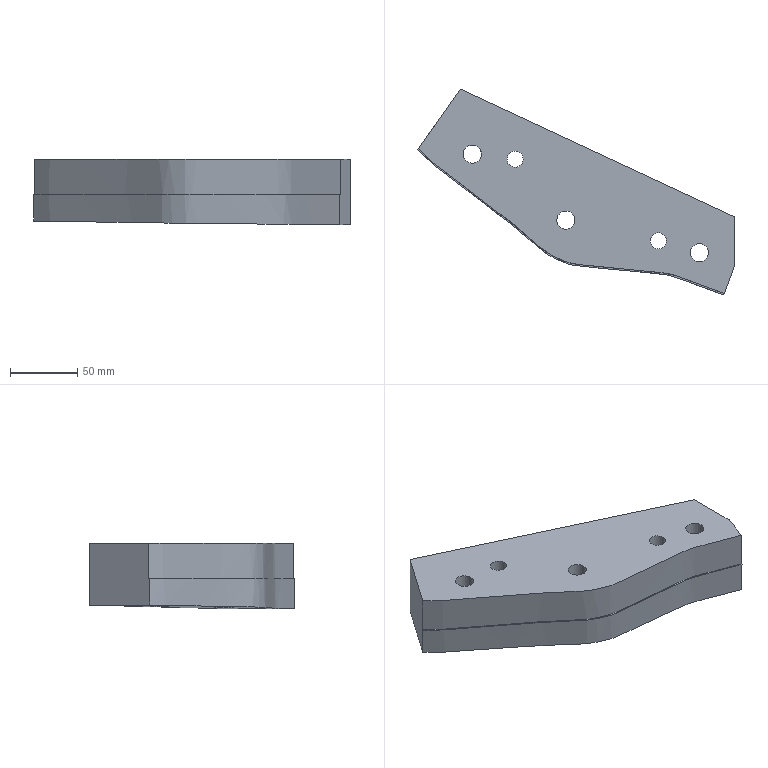Part | NX | features solid 2 | 1 solid | 24 faces | box 234.961 x 152.688 x 48.86 mm | volume 747452 mm3 | plane 12 | cylinder 10 | spline 2 | commonest cylinder face diameters 13.5 x3 19.5 x3 12 x2 13 x2
STEP:
#1=CARTESIAN_POINT('',(-144.165,133.045,40.));
#2=VERTEX_POINT('',#1);
#3=CARTESIAN_POINT('',(-150.915,133.045,40.));
#4=DIRECTION('',(0.,0.,1.));
#5=DIRECTION('',(1.,0.,0.));
#6=AXIS2_PLACEMENT_3D('',#3,#4,#5);
#7=CIRCLE('',#6,6.75);
#8=EDGE_CURVE('',#2,#2,#7,.T.);
#9=ORIENTED_EDGE('',*,*,#8,.F.);
#10=EDGE_LOOP('',(#9));
#11=FACE_BOUND('',#10,.T.);
#12=CARTESIAN_POINT('',(-312.729,206.131,40.));
#13=VERTEX_POINT('',#12);
#14=CARTESIAN_POINT('',(-319.479,206.131,40.));
#15=DIRECTION('',(0.,0.,1.));
#16=DIRECTION('',(1.,0.,0.));
#17=AXIS2_PLACEMENT_3D('',#14,#15,#16);
#18=CIRCLE('',#17,6.75);
#19=EDGE_CURVE('',#13,#13,#18,.T.);
#20=ORIENTED_EDGE('',*,*,#19,.F.);
#21=EDGE_LOOP('',(#20));
#22=FACE_BOUND('',#21,.T.);
#23=CARTESIAN_POINT('',(-243.241,157.177,40.));
#24=VERTEX_POINT('',#23);
#25=CARTESIAN_POINT('',(-249.991,157.177,40.));
#26=DIRECTION('',(0.,0.,1.));
#27=DIRECTION('',(1.,0.,0.));
#28=AXIS2_PLACEMENT_3D('',#25,#26,#27);
#29=CIRCLE('',#28,6.75);
#30=EDGE_CURVE('',#24,#24,#29,.T.);
#31=ORIENTED_EDGE('',*,*,#30,.F.);
#32=EDGE_LOOP('',(#31));
#33=FACE_BOUND('',#32,.T.);
#34=CARTESIAN_POINT('',(-175.436,141.76,40.));
#35=VERTEX_POINT('',#34);
#36=CARTESIAN_POINT('',(-181.436,141.76,40.));
#37=DIRECTION('',(0.,0.,1.));
#38=DIRECTION('',(1.,0.,0.));
#39=AXIS2_PLACEMENT_3D('',#36,#37,#38);
#40=CIRCLE('',#39,6.);
#41=EDGE_CURVE('',#35,#35,#40,.T.);
#42=ORIENTED_EDGE('',*,*,#41,.F.);
#43=EDGE_LOOP('',(#42));
#44=FACE_BOUND('',#43,.T.);
#45=CARTESIAN_POINT('',(-281.644,202.32,40.));
#46=VERTEX_POINT('',#45);
#47=CARTESIAN_POINT('',(-287.644,202.32,40.));
#48=DIRECTION('',(0.,0.,1.));
#49=DIRECTION('',(1.,0.,0.));
#50=AXIS2_PLACEMENT_3D('',#47,#48,#49);
#51=CIRCLE('',#50,6.);
#52=EDGE_CURVE('',#46,#46,#51,.T.);
#53=ORIENTED_EDGE('',*,*,#52,.F.);
#54=EDGE_LOOP('',(#53));
#55=FACE_BOUND('',#54,.T.);
#56=CARTESIAN_POINT('',(-132.408,102.674,40.));
#57=VERTEX_POINT('',#56);
#58=CARTESIAN_POINT('',(-359.384,210.162,40.));
#59=VERTEX_POINT('',#58);
#60=CARTESIAN_POINT('',(-132.408,102.674,40.));
#61=CARTESIAN_POINT('',(-133.704,103.14,40.));
#62=CARTESIAN_POINT('',(-136.335,104.003,40.));
#63=CARTESIAN_POINT('',(-141.52,105.911,40.));
#64=CARTESIAN_POINT('',(-147.98,108.359,40.));
#65=CARTESIAN_POINT('',(-155.752,111.253,40.));
#66=CARTESIAN_POINT('',(-163.506,114.139,40.));
#67=CARTESIAN_POINT('',(-171.267,117.226,40.));
#68=CARTESIAN_POINT('',(-179.47,118.263,40.));
#69=CARTESIAN_POINT('',(-187.623,119.24,40.));
#70=CARTESIAN_POINT('',(-195.819,119.959,40.));
#71=CARTESIAN_POINT('',(-204.02,120.604,40.));
#72=CARTESIAN_POINT('',(-212.219,121.277,40.));
#73=CARTESIAN_POINT('',(-220.405,122.065,40.));
#74=CARTESIAN_POINT('',(-228.561,123.135,40.));
#75=CARTESIAN_POINT('',(-235.386,123.797,40.));
#76=CARTESIAN_POINT('',(-240.845,124.247,40.));
#77=CARTESIAN_POINT('',(-244.943,124.767,40.));
#78=CARTESIAN_POINT('',(-248.867,125.792,40.));
#79=CARTESIAN_POINT('',(-252.61,127.306,40.));
#80=CARTESIAN_POINT('',(-256.299,128.954,40.));
#81=CARTESIAN_POINT('',(-259.983,130.668,40.));
#82=CARTESIAN_POINT('',(-263.483,132.667,40.));
#83=CARTESIAN_POINT('',(-266.659,135.061,40.));
#84=CARTESIAN_POINT('',(-269.686,137.645,40.));
#85=CARTESIAN_POINT('',(-272.75,140.183,40.));
#86=CARTESIAN_POINT('',(-275.752,142.798,40.));
#87=CARTESIAN_POINT('',(-279.678,146.382,40.));
#88=CARTESIAN_POINT('',(-284.663,150.764,40.));
#89=CARTESIAN_POINT('',(-290.913,155.686,40.));
#90=CARTESIAN_POINT('',(-299.232,162.266,40.));
#91=CARTESIAN_POINT('',(-309.703,170.4,40.));
#92=CARTESIAN_POINT('',(-320.302,178.373,40.));
#93=CARTESIAN_POINT('',(-328.787,184.744,40.));
#94=CARTESIAN_POINT('',(-335.144,189.531,40.));
#95=CARTESIAN_POINT('',(-341.443,194.391,40.));
#96=CARTESIAN_POINT('',(-346.778,198.333,40.));
#97=CARTESIAN_POINT('',(-350.821,201.768,40.));
#98=CARTESIAN_POINT('',(-354.614,205.514,40.));
#99=CARTESIAN_POINT('',(-357.386,208.414,40.));
#100=CARTESIAN_POINT('',(-359.384,210.162,40.));
#101=B_SPLINE_CURVE_WITH_KNOTS('',3,(#60,#61,#62,#63,#64,#65,#66,#67,#68,#69,#70,#71,#72,#73,#74,#75,#76,#77,#78,#79,#80,#81,#82,#83,#84,#85,#86,#87,#88,#89,#90,#91,#92,#93,#94,#95,#96,#97,#98,#99,#100),.UNSPECIFIED.,.F.,.F.,(4,1,1,1,1,1,1,1,1,1,1,1,1,1,1,1,1,1,1,1,1,1,1,1,1,1,1,1,1,1,1,1,1,1,1,1,1,1,4),(0.01102,0.01506,0.0191,0.02717,0.03525,0.04332,0.0514,0.05947,0.06755,0.07562,0.0837,0.09177,0.09985,0.1079,0.116,0.12,0.1241,0.1281,0.1322,0.1362,0.1402,0.1443,0.1483,0.1523,0.1564,0.1604,0.1645,0.1725,0.1806,0.1887,0.2048,0.221,0.2291,0.2371,0.2452,0.2533,0.2573,0.2614,0.2694),.UNSPECIFIED.);
#102=EDGE_CURVE('',#57,#59,#101,.T.);
#103=ORIENTED_EDGE('',*,*,#102,.F.);
#104=CARTESIAN_POINT('',(-125.,123.027,40.));
#105=VERTEX_POINT('',#104);
#106=CARTESIAN_POINT('',(-187.242,-47.981,40.));
#107=DIRECTION('',(0.342,0.9397,0.));
#108=VECTOR('',#107,1000.);
#109=LINE('',#106,#108);
#110=EDGE_CURVE('',#57,#105,#109,.T.);
#111=ORIENTED_EDGE('',*,*,#110,.T.);
#112=CARTESIAN_POINT('',(-125.,159.579,40.));
#113=VERTEX_POINT('',#112);
#114=CARTESIAN_POINT('',(-125.,35.09,40.));
#115=DIRECTION('',(0.,1.,0.));
#116=VECTOR('',#115,1000.);
#117=LINE('',#114,#116);
#118=EDGE_CURVE('',#105,#113,#117,.T.);
#119=ORIENTED_EDGE('',*,*,#118,.T.);
#120=CARTESIAN_POINT('',(-328.392,254.422,40.));
#121=VERTEX_POINT('',#120);
#122=CARTESIAN_POINT('',(-99.435,147.658,40.));
#123=DIRECTION('',(0.9063,-0.4226,0.));
#124=VECTOR('',#123,1000.);
#125=LINE('',#122,#124);
#126=EDGE_CURVE('',#113,#121,#125,.F.);
#127=ORIENTED_EDGE('',*,*,#126,.T.);
#128=CARTESIAN_POINT('',(-460.095,66.332,40.));
#129=DIRECTION('',(0.5736,0.8192,0.));
#130=VECTOR('',#129,1000.);
#131=LINE('',#128,#130);
#132=EDGE_CURVE('',#59,#121,#131,.T.);
#133=ORIENTED_EDGE('',*,*,#132,.F.);
#134=EDGE_LOOP('',(#103,#111,#119,#127,#133));
#135=FACE_BOUND('',#134,.T.);
#136=CARTESIAN_POINT('',(-415.478,35.09,40.));
#137=DIRECTION('',(0.,0.,1.));
#138=DIRECTION('',(1.,0.,0.));
#139=AXIS2_PLACEMENT_3D('',#136,#137,#138);
#140=PLANE('',#139);
#141=ADVANCED_FACE('',(#11,#22,#33,#44,#55,#135),#140,.T.);
#142=ORIENTED_EDGE('',*,*,#118,.F.);
#143=CARTESIAN_POINT('',(-125.,123.027,-8.793));
#144=VERTEX_POINT('',#143);
#145=CARTESIAN_POINT('',(-125.,123.027,23.));
#146=DIRECTION('',(0.,0.,-1.));
#147=VECTOR('',#146,1000.);
#148=LINE('',#145,#147);
#149=EDGE_CURVE('',#105,#144,#148,.T.);
#150=ORIENTED_EDGE('',*,*,#149,.T.);
#151=CARTESIAN_POINT('',(-125.,159.579,-8.551));
#152=VERTEX_POINT('',#151);
#153=CARTESIAN_POINT('',(-125.,163.829,-8.523));
#154=DIRECTION('',(0.,-1.,-0.00662));
#155=VECTOR('',#154,1000.);
#156=LINE('',#153,#155);
#157=EDGE_CURVE('',#152,#144,#156,.T.);
#158=ORIENTED_EDGE('',*,*,#157,.F.);
#159=CARTESIAN_POINT('',(-125.,159.579,2.));
#160=DIRECTION('',(0.,0.,-1.));
#161=VECTOR('',#160,1000.);
#162=LINE('',#159,#161);
#163=EDGE_CURVE('',#152,#113,#162,.F.);
#164=ORIENTED_EDGE('',*,*,#163,.T.);
#165=EDGE_LOOP('',(#142,#150,#158,#164));
#166=FACE_BOUND('',#165,.T.);
#167=CARTESIAN_POINT('',(-125.,163.62,23.));
#168=DIRECTION('',(1.,0.,0.));
#169=DIRECTION('',(0.,0.,-1.));
#170=AXIS2_PLACEMENT_3D('',#167,#168,#169);
#171=PLANE('',#170);
#172=ADVANCED_FACE('',(#166),#171,.T.);
#173=CARTESIAN_POINT('',(-359.961,209.338,-6.));
#174=VERTEX_POINT('',#173);
#175=CARTESIAN_POINT('',(-132.75,101.734,-8.86));
#176=VERTEX_POINT('',#175);
#177=CARTESIAN_POINT('',(-359.961,209.338,-6.));
#178=CARTESIAN_POINT('',(-357.935,207.556,-6.031));
#179=CARTESIAN_POINT('',(-355.147,204.621,-6.077));
#180=CARTESIAN_POINT('',(-351.299,200.848,-6.138));
#181=CARTESIAN_POINT('',(-347.183,197.387,-6.2));
#182=CARTESIAN_POINT('',(-341.764,193.377,-6.278));
#183=CARTESIAN_POINT('',(-335.365,188.443,-6.371));
#184=CARTESIAN_POINT('',(-328.907,183.583,-6.464));
#185=CARTESIAN_POINT('',(-320.289,177.113,-6.588));
#186=CARTESIAN_POINT('',(-309.528,169.009,-6.744));
#187=CARTESIAN_POINT('',(-298.9,160.735,-6.899));
#188=CARTESIAN_POINT('',(-290.451,154.045,-7.023));
#189=CARTESIAN_POINT('',(-284.11,149.034,-7.116));
#190=CARTESIAN_POINT('',(-278.12,143.567,-7.209));
#191=CARTESIAN_POINT('',(-273.048,139.115,-7.287));
#192=CARTESIAN_POINT('',(-268.899,135.674,-7.349));
#193=CARTESIAN_POINT('',(-265.799,133.078,-7.395));
#194=CARTESIAN_POINT('',(-262.422,130.844,-7.442));
#195=CARTESIAN_POINT('',(-258.768,128.97,-7.489));
#196=CARTESIAN_POINT('',(-254.985,127.275,-7.536));
#197=CARTESIAN_POINT('',(-251.21,125.617,-7.582));
#198=CARTESIAN_POINT('',(-247.364,124.283,-7.628));
#199=CARTESIAN_POINT('',(-243.399,123.523,-7.67));
#200=CARTESIAN_POINT('',(-239.361,123.116,-7.711));
#201=CARTESIAN_POINT('',(-233.956,122.673,-7.765));
#202=CARTESIAN_POINT('',(-227.235,121.95,-7.833));
#203=CARTESIAN_POINT('',(-219.201,120.928,-7.916));
#204=CARTESIAN_POINT('',(-211.135,120.181,-7.997));
#205=CARTESIAN_POINT('',(-203.059,119.526,-8.078));
#206=CARTESIAN_POINT('',(-194.982,118.887,-8.159));
#207=CARTESIAN_POINT('',(-186.909,118.159,-8.24));
#208=CARTESIAN_POINT('',(-178.885,117.187,-8.322));
#209=CARTESIAN_POINT('',(-172.138,116.282,-8.392));
#210=CARTESIAN_POINT('',(-167.026,114.447,-8.452));
#211=CARTESIAN_POINT('',(-161.971,112.515,-8.513));
#212=CARTESIAN_POINT('',(-155.633,110.135,-8.589));
#213=CARTESIAN_POINT('',(-148.018,107.308,-8.679));
#214=CARTESIAN_POINT('',(-141.69,104.906,-8.755));
#215=CARTESIAN_POINT('',(-136.604,103.039,-8.815));
#216=CARTESIAN_POINT('',(-134.025,102.193,-8.845));
#217=CARTESIAN_POINT('',(-132.75,101.734,-8.86));
#218=B_SPLINE_CURVE_WITH_KNOTS('',3,(#177,#178,#179,#180,#181,#182,#183,#184,#185,#186,#187,#188,#189,#190,#191,#192,#193,#194,#195,#196,#197,#198,#199,#200,#201,#202,#203,#204,#205,#206,#207,#208,#209,#210,#211,#212,#213,#214,#215,#216,#217),.UNSPECIFIED.,.F.,.F.,(4,1,1,1,1,1,1,1,1,1,1,1,1,1,1,1,1,1,1,1,1,1,1,1,1,1,1,1,1,1,1,1,1,1,1,1,1,1,4),(0.,0.008086,0.01213,0.01617,0.02426,0.03234,0.04043,0.04852,0.06469,0.08086,0.08895,0.09703,0.1051,0.1132,0.1172,0.1213,0.1253,0.1294,0.1334,0.1375,0.1415,0.1456,0.1496,0.1536,0.1617,0.1698,0.1779,0.186,0.1941,0.2022,0.2102,0.2183,0.2224,0.2264,0.2345,0.2426,0.2507,0.2547,0.2588),.UNSPECIFIED.);
#219=EDGE_CURVE('',#174,#176,#218,.T.);
#220=ORIENTED_EDGE('',*,*,#219,.T.);
#221=CARTESIAN_POINT('',(-132.75,101.734,14.));
#222=VERTEX_POINT('',#221);
#223=CARTESIAN_POINT('',(-132.75,101.734,2.42));
#224=DIRECTION('',(0.,0.,-1.));
#225=VECTOR('',#224,1000.);
#226=LINE('',#223,#225);
#227=EDGE_CURVE('',#176,#222,#226,.F.);
#228=ORIENTED_EDGE('',*,*,#227,.T.);
#229=CARTESIAN_POINT('',(-359.961,209.338,14.));
#230=VERTEX_POINT('',#229);
#231=CARTESIAN_POINT('',(-112.285,93.733,14.));
#232=CARTESIAN_POINT('',(-115.856,94.563,14.));
#233=CARTESIAN_POINT('',(-119.426,95.392,14.));
#234=CARTESIAN_POINT('',(-122.997,96.222,14.));
#235=CARTESIAN_POINT('',(-124.392,96.546,14.));
#236=CARTESIAN_POINT('',(-126.827,98.157,14.));
#237=CARTESIAN_POINT('',(-130.155,100.898,14.));
#238=CARTESIAN_POINT('',(-134.281,102.244,14.));
#239=CARTESIAN_POINT('',(-139.679,104.141,14.));
#240=CARTESIAN_POINT('',(-146.371,106.694,14.));
#241=CARTESIAN_POINT('',(-154.427,109.679,14.));
#242=CARTESIAN_POINT('',(-161.126,112.208,14.));
#243=CARTESIAN_POINT('',(-165.815,113.972,14.));
#244=CARTESIAN_POINT('',(-168.494,114.99,14.));
#245=CARTESIAN_POINT('',(-171.216,115.884,14.));
#246=CARTESIAN_POINT('',(-174.721,116.613,14.));
#247=CARTESIAN_POINT('',(-178.987,117.19,14.));
#248=CARTESIAN_POINT('',(-183.249,117.724,14.));
#249=CARTESIAN_POINT('',(-191.788,118.655,14.));
#250=CARTESIAN_POINT('',(-204.643,119.63,14.));
#251=CARTESIAN_POINT('',(-218.911,120.84,14.));
#252=CARTESIAN_POINT('',(-228.851,122.152,14.));
#253=CARTESIAN_POINT('',(-234.551,122.715,14.));
#254=CARTESIAN_POINT('',(-238.829,123.073,14.));
#255=CARTESIAN_POINT('',(-243.12,123.479,14.));
#256=CARTESIAN_POINT('',(-248.75,124.526,14.));
#257=CARTESIAN_POINT('',(-255.34,127.421,14.));
#258=CARTESIAN_POINT('',(-261.873,130.381,14.));
#259=CARTESIAN_POINT('',(-265.989,133.26,14.));
#260=CARTESIAN_POINT('',(-268.199,135.082,14.));
#261=CARTESIAN_POINT('',(-270.393,136.924,14.));
#262=CARTESIAN_POINT('',(-273.148,139.209,14.));
#263=CARTESIAN_POINT('',(-277.472,142.965,14.));
#264=CARTESIAN_POINT('',(-282.708,147.853,14.));
#265=CARTESIAN_POINT('',(-289.411,153.233,14.));
#266=CARTESIAN_POINT('',(-298.398,160.336,14.));
#267=CARTESIAN_POINT('',(-314.207,172.665,14.));
#268=CARTESIAN_POINT('',(-330.339,184.575,14.));
#269=CARTESIAN_POINT('',(-343.963,195.04,14.));
#270=CARTESIAN_POINT('',(-350.855,200.194,14.));
#271=CARTESIAN_POINT('',(-355.804,205.388,14.));
#272=CARTESIAN_POINT('',(-359.395,208.889,14.));
#273=CARTESIAN_POINT('',(-361.592,210.724,14.));
#274=CARTESIAN_POINT('',(-363.291,212.042,14.));
#275=CARTESIAN_POINT('',(-364.964,213.384,14.));
#276=CARTESIAN_POINT('',(-366.621,214.773,14.));
#277=CARTESIAN_POINT('',(-368.75,215.407,14.));
#278=CARTESIAN_POINT('',(-370.894,214.756,14.));
#279=CARTESIAN_POINT('',(-372.124,213.383,14.));
#280=CARTESIAN_POINT('',(-372.711,212.074,14.));
#281=CARTESIAN_POINT('',(-373.494,210.073,14.));
#282=CARTESIAN_POINT('',(-374.087,207.63,14.));
#283=CARTESIAN_POINT('',(-375.074,204.941,14.));
#284=CARTESIAN_POINT('',(-375.964,202.22,14.));
#285=CARTESIAN_POINT('',(-377.061,198.808,14.));
#286=CARTESIAN_POINT('',(-378.358,194.734,14.));
#287=CARTESIAN_POINT('',(-379.476,191.261,14.));
#288=CARTESIAN_POINT('',(-381.61,189.247,14.));
#289=CARTESIAN_POINT('',(-384.401,188.338,14.));
#290=CARTESIAN_POINT('',(-387.982,189.153,14.));
#291=CARTESIAN_POINT('',(-392.089,190.337,14.));
#292=CARTESIAN_POINT('',(-397.637,191.766,14.));
#293=CARTESIAN_POINT('',(-402.142,192.907,14.));
#294=CARTESIAN_POINT('',(-405.767,193.016,14.));
#295=CARTESIAN_POINT('',(-406.752,192.482,14.));
#296=CARTESIAN_POINT('',(-407.204,191.679,14.));
#297=CARTESIAN_POINT('',(-407.355,190.978,14.));
#298=CARTESIAN_POINT('',(-407.778,189.239,14.));
#299=CARTESIAN_POINT('',(-409.476,182.099,14.));
#300=CARTESIAN_POINT('',(-411.921,172.376,14.));
#301=CARTESIAN_POINT('',(-414.76,162.76,14.));
#302=CARTESIAN_POINT('',(-416.63,157.346,14.));
#303=CARTESIAN_POINT('',(-418.178,153.337,14.));
#304=CARTESIAN_POINT('',(-420.236,149.537,14.));
#305=CARTESIAN_POINT('',(-423.236,146.416,14.));
#306=CARTESIAN_POINT('',(-426.787,143.984,14.));
#307=CARTESIAN_POINT('',(-431.478,140.7,14.));
#308=CARTESIAN_POINT('',(-437.23,136.434,14.));
#309=CARTESIAN_POINT('',(-444.283,131.521,14.));
#310=CARTESIAN_POINT('',(-450.102,127.369,14.));
#311=CARTESIAN_POINT('',(-454.183,123.24,14.));
#312=CARTESIAN_POINT('',(-456.026,120.178,14.));
#313=CARTESIAN_POINT('',(-456.869,117.432,14.));
#314=CARTESIAN_POINT('',(-457.557,114.647,14.));
#315=CARTESIAN_POINT('',(-458.426,111.177,14.));
#316=CARTESIAN_POINT('',(-459.295,107.705,14.));
#317=CARTESIAN_POINT('',(-460.068,104.944,14.));
#318=CARTESIAN_POINT('',(-460.556,102.852,14.));
#319=CARTESIAN_POINT('',(-460.759,100.705,14.));
#320=CARTESIAN_POINT('',(-460.539,97.842,14.));
#321=CARTESIAN_POINT('',(-458.816,93.054,14.));
#322=CARTESIAN_POINT('',(-454.37,88.976,14.));
#323=CARTESIAN_POINT('',(-449.483,87.695,14.));
#324=CARTESIAN_POINT('',(-446.657,87.236,14.));
#325=CARTESIAN_POINT('',(-443.828,86.787,14.));
#326=CARTESIAN_POINT('',(-440.31,86.125,14.));
#327=CARTESIAN_POINT('',(-434.679,85.08,14.));
#328=CARTESIAN_POINT('',(-427.604,83.939,14.));
#329=CARTESIAN_POINT('',(-420.684,82.057,14.));
#330=CARTESIAN_POINT('',(-415.851,80.778,14.));
#331=CARTESIAN_POINT('',(-413.367,80.304,14.));
#332=CARTESIAN_POINT('',(-412.158,79.475,14.));
#333=CARTESIAN_POINT('',(-411.532,78.587,14.));
#334=CARTESIAN_POINT('',(-411.333,77.527,14.));
#335=CARTESIAN_POINT('',(-411.398,76.071,14.));
#336=CARTESIAN_POINT('',(-411.844,73.616,14.));
#337=CARTESIAN_POINT('',(-412.388,68.624,14.));
#338=CARTESIAN_POINT('',(-413.428,61.542,14.));
#339=CARTESIAN_POINT('',(-414.451,50.13,14.));
#340=CARTESIAN_POINT('',(-415.942,30.138,14.));
#341=CARTESIAN_POINT('',(-416.835,1.497,14.));
#342=CARTESIAN_POINT('',(-415.947,-27.14,14.));
#343=CARTESIAN_POINT('',(-414.318,-47.126,14.));
#344=CARTESIAN_POINT('',(-413.277,-56.375,14.));
#345=CARTESIAN_POINT('',(-412.75,-60.639,14.));
#346=CARTESIAN_POINT('',(-412.511,-62.774,14.));
#347=CARTESIAN_POINT('',(-412.138,-64.888,14.));
#348=CARTESIAN_POINT('',(-411.199,-69.083,14.));
#349=CARTESIAN_POINT('',(-410.509,-72.962,14.));
#350=CARTESIAN_POINT('',(-409.724,-76.453,14.));
#351=CARTESIAN_POINT('',(-409.446,-77.862,14.));
#352=CARTESIAN_POINT('',(-409.727,-79.695,14.));
#353=CARTESIAN_POINT('',(-410.96,-81.089,14.));
#354=CARTESIAN_POINT('',(-412.257,-81.717,14.));
#355=CARTESIAN_POINT('',(-414.338,-82.265,14.));
#356=CARTESIAN_POINT('',(-417.449,-83.095,14.));
#357=CARTESIAN_POINT('',(-422.943,-84.715,14.));
#358=CARTESIAN_POINT('',(-429.89,-86.483,14.));
#359=CARTESIAN_POINT('',(-438.395,-87.724,14.));
#360=CARTESIAN_POINT('',(-445.478,-88.761,14.));
#361=CARTESIAN_POINT('',(-451.053,-90.196,14.));
#362=CARTESIAN_POINT('',(-456.021,-93.16,14.));
#363=CARTESIAN_POINT('',(-460.459,-99.179,14.));
#364=CARTESIAN_POINT('',(-460.609,-106.618,14.));
#365=CARTESIAN_POINT('',(-458.817,-112.069,14.));
#366=CARTESIAN_POINT('',(-457.691,-116.214,14.));
#367=CARTESIAN_POINT('',(-456.643,-120.377,14.));
#368=CARTESIAN_POINT('',(-454.688,-125.83,14.));
#369=CARTESIAN_POINT('',(-450.288,-129.768,14.));
#370=CARTESIAN_POINT('',(-446.15,-132.56,14.));
#371=CARTESIAN_POINT('',(-443.768,-134.151,14.));
#372=CARTESIAN_POINT('',(-441.987,-135.352,14.));
#373=CARTESIAN_POINT('',(-440.183,-136.518,14.));
#374=CARTESIAN_POINT('',(-437.722,-137.982,14.));
#375=CARTESIAN_POINT('',(-434.578,-139.696,14.));
#376=CARTESIAN_POINT('',(-431.016,-142.118,14.));
#377=CARTESIAN_POINT('',(-427.923,-145.11,14.));
#378=CARTESIAN_POINT('',(-425.28,-147.528,14.));
#379=CARTESIAN_POINT('',(-422.996,-149.255,14.));
#380=CARTESIAN_POINT('',(-420.694,-150.963,14.));
#381=CARTESIAN_POINT('',(-418.103,-153.445,14.));
#382=CARTESIAN_POINT('',(-414.699,-158.081,14.));
#383=CARTESIAN_POINT('',(-411.818,-164.69,14.));
#384=CARTESIAN_POINT('',(-409.69,-173.02,14.));
#385=CARTESIAN_POINT('',(-407.349,-181.283,14.));
#386=CARTESIAN_POINT('',(-405.436,-188.189,14.));
#387=CARTESIAN_POINT('',(-404.277,-192.687,14.));
#388=CARTESIAN_POINT('',(-403.731,-194.774,14.));
#389=CARTESIAN_POINT('',(-402.911,-195.983,14.));
#390=CARTESIAN_POINT('',(-401.476,-196.55,14.));
#391=CARTESIAN_POINT('',(-400.058,-196.272,14.));
#392=CARTESIAN_POINT('',(-398.677,-195.897,14.));
#393=CARTESIAN_POINT('',(-396.258,-195.238,14.));
#394=CARTESIAN_POINT('',(-392.822,-194.236,14.));
#395=CARTESIAN_POINT('',(-389.356,-193.338,14.));
#396=CARTESIAN_POINT('',(-386.595,-192.576,14.));
#397=CARTESIAN_POINT('',(-383.879,-191.694,14.));
#398=CARTESIAN_POINT('',(-381.029,-191.005,14.));
#399=CARTESIAN_POINT('',(-378.195,-191.605,14.));
#400=CARTESIAN_POINT('',(-375.647,-193.039,14.));
#401=CARTESIAN_POINT('',(-373.775,-196.061,14.));
#402=CARTESIAN_POINT('',(-372.459,-200.297,14.));
#403=CARTESIAN_POINT('',(-370.755,-204.215,14.));
#404=CARTESIAN_POINT('',(-369.584,-207.601,14.));
#405=CARTESIAN_POINT('',(-368.811,-210.358,14.));
#406=CARTESIAN_POINT('',(-368.284,-212.445,14.));
#407=CARTESIAN_POINT('',(-367.403,-214.035,14.));
#408=CARTESIAN_POINT('',(-366.332,-215.009,14.));
#409=CARTESIAN_POINT('',(-364.997,-215.589,14.));
#410=CARTESIAN_POINT('',(-363.147,-215.431,14.));
#411=CARTESIAN_POINT('',(-361.272,-214.331,14.));
#412=CARTESIAN_POINT('',(-359.608,-212.974,14.));
#413=CARTESIAN_POINT('',(-356.215,-210.34,14.));
#414=CARTESIAN_POINT('',(-349.028,-204.423,14.));
#415=CARTESIAN_POINT('',(-337.771,-195.573,14.));
#416=CARTESIAN_POINT('',(-324.236,-184.984,14.));
#417=CARTESIAN_POINT('',(-313.055,-176.037,14.));
#418=CARTESIAN_POINT('',(-304.322,-168.623,14.));
#419=CARTESIAN_POINT('',(-297.827,-162.998,14.));
#420=CARTESIAN_POINT('',(-291.244,-157.477,14.));
#421=CARTESIAN_POINT('',(-284.555,-152.085,14.));
#422=CARTESIAN_POINT('',(-277.805,-146.768,14.));
#423=CARTESIAN_POINT('',(-271.113,-141.381,14.));
#424=CARTESIAN_POINT('',(-264.538,-135.852,14.));
#425=CARTESIAN_POINT('',(-257.668,-130.656,14.));
#426=CARTESIAN_POINT('',(-251.187,-127.53,14.));
#427=CARTESIAN_POINT('',(-245.74,-125.755,14.));
#428=CARTESIAN_POINT('',(-241.581,-124.657,14.));
#429=CARTESIAN_POINT('',(-237.367,-123.812,14.));
#430=CARTESIAN_POINT('',(-231.672,-123.168,14.));
#431=CARTESIAN_POINT('',(-224.501,-123.191,14.));
#432=CARTESIAN_POINT('',(-215.929,-122.567,14.));
#433=CARTESIAN_POINT('',(-208.768,-122.461,14.));
#434=CARTESIAN_POINT('',(-203.041,-122.532,14.));
#435=CARTESIAN_POINT('',(-198.743,-122.639,14.));
#436=CARTESIAN_POINT('',(-194.457,-122.273,14.));
#437=CARTESIAN_POINT('',(-191.639,-121.752,14.));
#438=CARTESIAN_POINT('',(-190.231,-121.49,14.));
#439=B_SPLINE_CURVE_WITH_KNOTS('',3,(#231,#232,#233,#234,#235,#236,#237,#238,#239,#240,#241,#242,#243,#244,#245,#246,#247,#248,#249,#250,#251,#252,#253,#254,#255,#256,#257,#258,#259,#260,#261,#262,#263,#264,#265,#266,#267,#268,#269,#270,#271,#272,#273,#274,#275,#276,#277,#278,#279,#280,#281,#282,#283,#284,#285,#286,#287,#288,#289,#290,#291,#292,#293,#294,#295,#296,#297,#298,#299,#300,#301,#302,#303,#304,#305,#306,#307,#308,#309,#310,#311,#312,#313,#314,#315,#316,#317,#318,#319,#320,#321,#322,#323,#324,#325,#326,#327,#328,#329,#330,#331,#332,#333,#334,#335,#336,#337,#338,#339,#340,#341,#342,#343,#344,#345,#346,#347,#348,#349,#350,#351,#352,#353,#354,#355,#356,#357,#358,#359,#360,#361,#362,#363,#364,#365,#366,#367,#368,#369,#370,#371,#372,#373,#374,#375,#376,#377,#378,#379,#380,#381,#382,#383,#384,#385,#386,#387,#388,#389,#390,#391,#392,#393,#394,#395,#396,#397,#398,#399,#400,#401,#402,#403,#404,#405,#406,#407,#408,#409,#410,#411,#412,#413,#414,#415,#416,#417,#418,#419,#420,#421,#422,#423,#424,#425,#426,#427,#428,#429,#430,#431,#432,#433,#434,#435,#436,#437,#438),.UNSPECIFIED.,.F.,.F.,(4,3,1,1,1,1,1,1,1,1,1,1,1,1,1,1,1,1,1,1,1,1,1,1,1,1,1,1,1,1,1,1,1,1,1,1,1,1,1,1,1,1,1,1,1,1,1,1,1,1,1,1,1,1,1,1,1,1,1,1,1,1,1,1,1,1,1,1,1,1,1,1,1,1,1,1,1,1,1,1,1,1,1,1,1,1,1,1,1,1,1,1,1,1,1,1,1,1,1,1,1,1,1,1,1,1,1,1,1,1,1,1,1,1,1,1,1,1,1,1,1,1,1,1,1,1,1,1,1,1,1,1,1,1,1,1,1,1,1,1,1,1,1,1,1,1,1,1,1,1,1,1,1,1,1,1,1,1,1,1,1,1,1,1,1,1,1,1,1,1,1,1,1,1,1,1,1,1,1,1,1,1,1,1,1,1,1,1,1,1,1,1,1,1,1,1,1,1,1,1,1,1,1,4),(-0.004704,0.,0.001837,0.003675,0.005512,0.007349,0.01102,0.0147,0.01837,0.02021,0.02113,0.02205,0.02388,0.02572,0.02756,0.0294,0.03675,0.0441,0.04777,0.04961,0.05144,0.05328,0.05512,0.05879,0.06247,0.06431,0.06522,0.06614,0.06798,0.06982,0.07349,0.07717,0.08084,0.08819,0.1029,0.1066,0.1102,0.1139,0.1158,0.1167,0.1176,0.1185,0.1194,0.1203,0.1213,0.1222,0.1226,0.1231,0.1249,0.1259,0.1268,0.1286,0.1304,0.1323,0.1332,0.1341,0.136,0.1378,0.1396,0.1433,0.1438,0.1442,0.1447,0.1449,0.1451,0.147,0.1543,0.158,0.1598,0.1617,0.1635,0.1654,0.1672,0.169,0.1727,0.1764,0.1801,0.1819,0.1837,0.1846,0.1856,0.1874,0.1892,0.1902,0.1911,0.192,0.1929,0.1948,0.1984,0.2003,0.2012,0.2021,0.2039,0.2058,0.2095,0.2131,0.215,0.2159,0.2163,0.2168,0.2173,0.2177,0.2186,0.2205,0.2242,0.2278,0.2352,0.2499,0.2646,0.2719,0.2756,0.2765,0.2774,0.2784,0.2793,0.2829,0.2834,0.2839,0.2848,0.2857,0.2862,0.2866,0.2885,0.2903,0.294,0.2976,0.3013,0.3032,0.305,0.3087,0.3123,0.3142,0.316,0.3179,0.3197,0.3234,0.3252,0.3261,0.327,0.328,0.3289,0.3307,0.3326,0.3344,0.3362,0.3371,0.3381,0.3399,0.3417,0.3454,0.3491,0.3528,0.3564,0.3583,0.3587,0.3592,0.3601,0.3606,0.361,0.3619,0.3638,0.3656,0.3665,0.3675,0.3693,0.3702,0.3711,0.373,0.3748,0.3766,0.3785,0.3794,0.3803,0.3812,0.3817,0.3822,0.3831,0.384,0.3849,0.3858,0.3895,0.3969,0.4042,0.4116,0.4152,0.4189,0.4226,0.4263,0.4299,0.4336,0.4373,0.441,0.4446,0.4465,0.4483,0.4501,0.452,0.4557,0.4593,0.463,0.4648,0.4667,0.4685,0.4704),.UNSPECIFIED.);
#440=EDGE_CURVE('',#230,#222,#439,.F.);
#441=ORIENTED_EDGE('',*,*,#440,.F.);
#442=CARTESIAN_POINT('',(-359.961,209.338,4.));
#443=DIRECTION('',(0.,0.,-1.));
#444=VECTOR('',#443,1000.);
#445=LINE('',#442,#444);
#446=EDGE_CURVE('',#174,#230,#445,.F.);
#447=ORIENTED_EDGE('',*,*,#446,.F.);
#448=EDGE_LOOP('',(#220,#228,#441,#447));
#449=FACE_BOUND('',#448,.T.);
#450=CARTESIAN_POINT('',(-132.75,101.734,14.));
#451=CARTESIAN_POINT('',(-132.75,101.734,-8.998));
#452=CARTESIAN_POINT('',(-134.025,102.193,14.));
#453=CARTESIAN_POINT('',(-134.025,102.193,-8.998));
#454=CARTESIAN_POINT('',(-136.604,103.039,14.));
#455=CARTESIAN_POINT('',(-136.604,103.039,-8.998));
#456=CARTESIAN_POINT('',(-141.668,104.898,14.));
#457=CARTESIAN_POINT('',(-141.668,104.898,-8.998));
#458=CARTESIAN_POINT('',(-147.987,107.296,14.));
#459=CARTESIAN_POINT('',(-147.987,107.296,-8.998));
#460=CARTESIAN_POINT('',(-155.584,110.116,14.));
#461=CARTESIAN_POINT('',(-155.584,110.116,-8.998));
#462=CARTESIAN_POINT('',(-161.907,112.493,14.));
#463=CARTESIAN_POINT('',(-161.907,112.493,-8.998));
#464=CARTESIAN_POINT('',(-166.954,114.418,14.));
#465=CARTESIAN_POINT('',(-166.954,114.418,-8.998));
#466=CARTESIAN_POINT('',(-172.044,116.259,14.));
#467=CARTESIAN_POINT('',(-172.044,116.259,-8.998));
#468=CARTESIAN_POINT('',(-178.771,117.175,14.));
#469=CARTESIAN_POINT('',(-178.771,117.175,-8.998));
#470=CARTESIAN_POINT('',(-186.807,118.147,14.));
#471=CARTESIAN_POINT('',(-186.807,118.147,-8.998));
#472=CARTESIAN_POINT('',(-194.88,118.879,14.));
#473=CARTESIAN_POINT('',(-194.88,118.879,-8.998));
#474=CARTESIAN_POINT('',(-202.961,119.519,14.));
#475=CARTESIAN_POINT('',(-202.961,119.519,-8.998));
#476=CARTESIAN_POINT('',(-211.041,120.173,14.));
#477=CARTESIAN_POINT('',(-211.041,120.173,-8.998));
#478=CARTESIAN_POINT('',(-219.11,120.919,14.));
#479=CARTESIAN_POINT('',(-219.11,120.919,-8.998));
#480=CARTESIAN_POINT('',(-227.152,121.939,14.));
#481=CARTESIAN_POINT('',(-227.152,121.939,-8.998));
#482=CARTESIAN_POINT('',(-233.866,122.665,14.));
#483=CARTESIAN_POINT('',(-233.866,122.665,-8.998));
#484=CARTESIAN_POINT('',(-239.25,123.107,14.));
#485=CARTESIAN_POINT('',(-239.25,123.107,-8.998));
#486=CARTESIAN_POINT('',(-243.296,123.509,14.));
#487=CARTESIAN_POINT('',(-243.296,123.509,-8.998));
#488=CARTESIAN_POINT('',(-247.276,124.259,14.));
#489=CARTESIAN_POINT('',(-247.276,124.259,-8.998));
#490=CARTESIAN_POINT('',(-251.098,125.572,14.));
#491=CARTESIAN_POINT('',(-251.098,125.572,-8.998));
#492=CARTESIAN_POINT('',(-254.825,127.203,14.));
#493=CARTESIAN_POINT('',(-254.825,127.203,-8.998));
#494=CARTESIAN_POINT('',(-258.536,128.864,14.));
#495=CARTESIAN_POINT('',(-258.536,128.864,-8.998));
#496=CARTESIAN_POINT('',(-262.147,130.689,14.));
#497=CARTESIAN_POINT('',(-262.147,130.689,-8.998));
#498=CARTESIAN_POINT('',(-265.553,132.892,14.));
#499=CARTESIAN_POINT('',(-265.553,132.892,-8.998));
#500=CARTESIAN_POINT('',(-268.676,135.482,14.));
#501=CARTESIAN_POINT('',(-268.676,135.482,-8.998));
#502=CARTESIAN_POINT('',(-272.829,138.937,14.));
#503=CARTESIAN_POINT('',(-272.829,138.937,-8.998));
#504=CARTESIAN_POINT('',(-277.92,143.376,14.));
#505=CARTESIAN_POINT('',(-277.92,143.376,-8.998));
#506=CARTESIAN_POINT('',(-283.894,148.855,14.));
#507=CARTESIAN_POINT('',(-283.894,148.855,-8.998));
#508=CARTESIAN_POINT('',(-290.252,153.888,14.));
#509=CARTESIAN_POINT('',(-290.252,153.888,-8.998));
#510=CARTESIAN_POINT('',(-298.724,160.596,14.));
#511=CARTESIAN_POINT('',(-298.724,160.596,-8.998));
#512=CARTESIAN_POINT('',(-309.381,168.897,14.));
#513=CARTESIAN_POINT('',(-309.381,168.897,-8.998));
#514=CARTESIAN_POINT('',(-320.171,177.025,14.));
#515=CARTESIAN_POINT('',(-320.171,177.025,-8.998));
#516=CARTESIAN_POINT('',(-328.813,183.513,14.));
#517=CARTESIAN_POINT('',(-328.813,183.513,-8.998));
#518=CARTESIAN_POINT('',(-335.29,188.386,14.));
#519=CARTESIAN_POINT('',(-335.29,188.386,-8.998));
#520=CARTESIAN_POINT('',(-341.705,193.332,14.));
#521=CARTESIAN_POINT('',(-341.705,193.332,-8.998));
#522=CARTESIAN_POINT('',(-347.144,197.357,14.));
#523=CARTESIAN_POINT('',(-347.144,197.357,-8.998));
#524=CARTESIAN_POINT('',(-351.277,200.827,14.));
#525=CARTESIAN_POINT('',(-351.277,200.827,-8.998));
#526=CARTESIAN_POINT('',(-355.134,204.607,14.));
#527=CARTESIAN_POINT('',(-355.134,204.607,-8.998));
#528=CARTESIAN_POINT('',(-357.933,207.555,14.));
#529=CARTESIAN_POINT('',(-357.933,207.555,-8.998));
#530=CARTESIAN_POINT('',(-359.961,209.338,14.));
#531=CARTESIAN_POINT('',(-359.961,209.338,-8.998));
#532=B_SPLINE_SURFACE_WITH_KNOTS('',3,1,((#450,#451),(#452,#453),(#454,#455),(#456,#457),(#458,#459),(#460,#461),(#462,#463),(#464,#465),(#466,#467),(#468,#469),(#470,#471),(#472,#473),(#474,#475),(#476,#477),(#478,#479),(#480,#481),(#482,#483),(#484,#485),(#486,#487),(#488,#489),(#490,#491),(#492,#493),(#494,#495),(#496,#497),(#498,#499),(#500,#501),(#502,#503),(#504,#505),(#506,#507),(#508,#509),(#510,#511),(#512,#513),(#514,#515),(#516,#517),(#518,#519),(#520,#521),(#522,#523),(#524,#525),(#526,#527),(#528,#529),(#530,#531)),.SURF_OF_LINEAR_EXTRUSION.,.F.,.F.,.F.,(4,1,1,1,1,1,1,1,1,1,1,1,1,1,1,1,1,1,1,1,1,1,1,1,1,1,1,1,1,1,1,1,1,1,1,1,1,1,4),(2,2),(0.004829,0.006562,0.008295,0.01176,0.01523,0.01869,0.02043,0.02216,0.02563,0.02909,0.03256,0.03603,0.03949,0.04296,0.04643,0.04989,0.05162,0.05336,0.05509,0.05682,0.05856,0.06029,0.06202,0.06376,0.06549,0.06722,0.07069,0.07416,0.07762,0.08109,0.08802,0.09495,0.09842,0.1019,0.1054,0.1088,0.1106,0.1123,0.1158),(0.,1.),.UNSPECIFIED.);
#533=ADVANCED_FACE('',(#449),#532,.T.);
#534=CARTESIAN_POINT('',(-282.32,198.592,-6.805));
#535=VERTEX_POINT('',#534);
#536=CARTESIAN_POINT('',(-287.644,202.32,-6.73));
#537=DIRECTION('',(0.009454,-0.00662,0.9999));
#538=DIRECTION('',(0.8191,-0.5735,-0.01154));
#539=AXIS2_PLACEMENT_3D('',#536,#537,#538);
#540=ELLIPSE('',#539,6.5,6.5);
#541=EDGE_CURVE('',#535,#535,#540,.T.);
#542=ORIENTED_EDGE('',*,*,#541,.T.);
#543=EDGE_LOOP('',(#542));
#544=FACE_BOUND('',#543,.T.);
#545=CARTESIAN_POINT('',(-176.111,138.032,-8.21));
#546=VERTEX_POINT('',#545);
#547=CARTESIAN_POINT('',(-181.436,141.76,-8.135));
#548=DIRECTION('',(0.009454,-0.00662,0.9999));
#549=DIRECTION('',(0.8191,-0.5735,-0.01154));
#550=AXIS2_PLACEMENT_3D('',#547,#548,#549);
#551=ELLIPSE('',#550,6.5,6.5);
#552=EDGE_CURVE('',#546,#546,#551,.T.);
#553=ORIENTED_EDGE('',*,*,#552,.T.);
#554=EDGE_LOOP('',(#553));
#555=FACE_BOUND('',#554,.T.);
#556=CARTESIAN_POINT('',(-242.004,151.585,-7.498));
#557=VERTEX_POINT('',#556);
#558=CARTESIAN_POINT('',(-249.991,157.177,-7.385));
#559=DIRECTION('',(0.009454,-0.00662,0.9999));
#560=DIRECTION('',(0.8191,-0.5735,-0.01154));
#561=AXIS2_PLACEMENT_3D('',#558,#559,#560);
#562=ELLIPSE('',#561,9.751,9.75);
#563=EDGE_CURVE('',#557,#557,#562,.T.);
#564=ORIENTED_EDGE('',*,*,#563,.T.);
#565=EDGE_LOOP('',(#564));
#566=FACE_BOUND('',#565,.T.);
#567=CARTESIAN_POINT('',(-311.492,200.539,-6.516));
#568=VERTEX_POINT('',#567);
#569=CARTESIAN_POINT('',(-319.479,206.131,-6.404));
#570=DIRECTION('',(0.009454,-0.00662,0.9999));
#571=DIRECTION('',(0.8191,-0.5735,-0.01154));
#572=AXIS2_PLACEMENT_3D('',#569,#570,#571);
#573=ELLIPSE('',#572,9.751,9.75);
#574=EDGE_CURVE('',#568,#568,#573,.T.);
#575=ORIENTED_EDGE('',*,*,#574,.T.);
#576=EDGE_LOOP('',(#575));
#577=FACE_BOUND('',#576,.T.);
#578=CARTESIAN_POINT('',(-142.928,127.453,-8.594));
#579=VERTEX_POINT('',#578);
#580=CARTESIAN_POINT('',(-150.915,133.045,-8.481));
#581=DIRECTION('',(0.009454,-0.00662,0.9999));
#582=DIRECTION('',(0.8191,-0.5735,-0.01154));
#583=AXIS2_PLACEMENT_3D('',#580,#581,#582);
#584=ELLIPSE('',#583,9.751,9.75);
#585=EDGE_CURVE('',#579,#579,#584,.T.);
#586=ORIENTED_EDGE('',*,*,#585,.T.);
#587=EDGE_LOOP('',(#586));
#588=FACE_BOUND('',#587,.T.);
#589=CARTESIAN_POINT('',(-109.914,164.474,-8.661));
#590=DIRECTION('',(0.342,0.9397,0.002987));
#591=VECTOR('',#590,1000.);
#592=LINE('',#589,#591);
#593=EDGE_CURVE('',#176,#144,#592,.T.);
#594=ORIENTED_EDGE('',*,*,#593,.F.);
#595=ORIENTED_EDGE('',*,*,#219,.F.);
#596=CARTESIAN_POINT('',(-328.392,254.422,-6.));
#597=VERTEX_POINT('',#596);
#598=CARTESIAN_POINT('',(-598.95,-131.975,-6.));
#599=DIRECTION('',(-0.5736,-0.8192,0.));
#600=VECTOR('',#599,1000.);
#601=LINE('',#598,#600);
#602=EDGE_CURVE('',#597,#174,#601,.T.);
#603=ORIENTED_EDGE('',*,*,#602,.F.);
#604=CARTESIAN_POINT('',(-329.99,255.167,-5.98));
#605=DIRECTION('',(-0.9062,0.4226,0.01137));
#606=VECTOR('',#605,1000.);
#607=LINE('',#604,#606);
#608=EDGE_CURVE('',#597,#152,#607,.F.);
#609=ORIENTED_EDGE('',*,*,#608,.T.);
#610=ORIENTED_EDGE('',*,*,#157,.T.);
#611=EDGE_LOOP('',(#594,#595,#603,#609,#610));
#612=FACE_BOUND('',#611,.T.);
#613=CARTESIAN_POINT('',(-334.216,246.104,-6.));
#614=DIRECTION('',(0.009454,-0.00662,0.9999));
#615=DIRECTION('',(1.,0.,-0.009454));
#616=AXIS2_PLACEMENT_3D('',#613,#614,#615);
#617=PLANE('',#616);
#618=ADVANCED_FACE('',(#544,#555,#566,#577,#588,#612),#617,.F.);
#619=CARTESIAN_POINT('',(-132.408,102.674,14.));
#620=VERTEX_POINT('',#619);
#621=CARTESIAN_POINT('',(-211.217,-113.852,14.));
#622=DIRECTION('',(-0.342,-0.9397,0.));
#623=VECTOR('',#622,1000.);
#624=LINE('',#621,#623);
#625=EDGE_CURVE('',#620,#222,#624,.T.);
#626=ORIENTED_EDGE('',*,*,#625,.F.);
#627=CARTESIAN_POINT('',(-359.384,210.162,14.));
#628=VERTEX_POINT('',#627);
#629=CARTESIAN_POINT('',(-132.408,102.674,14.));
#630=CARTESIAN_POINT('',(-133.72,103.146,14.));
#631=CARTESIAN_POINT('',(-136.262,103.978,14.));
#632=CARTESIAN_POINT('',(-141.317,105.835,14.));
#633=CARTESIAN_POINT('',(-147.641,108.234,14.));
#634=CARTESIAN_POINT('',(-155.235,111.053,14.));
#635=CARTESIAN_POINT('',(-161.577,113.437,14.));
#636=CARTESIAN_POINT('',(-166.59,115.348,14.));
#637=CARTESIAN_POINT('',(-170.514,116.773,14.));
#638=CARTESIAN_POINT('',(-174.604,117.6,14.));
#639=CARTESIAN_POINT('',(-180.004,118.341,14.));
#640=CARTESIAN_POINT('',(-186.725,119.141,14.));
#641=CARTESIAN_POINT('',(-194.822,119.879,14.));
#642=CARTESIAN_POINT('',(-202.911,120.518,14.));
#643=CARTESIAN_POINT('',(-210.987,121.172,14.));
#644=CARTESIAN_POINT('',(-219.04,121.917,14.));
#645=CARTESIAN_POINT('',(-227.056,122.935,14.));
#646=CARTESIAN_POINT('',(-233.819,123.665,14.));
#647=CARTESIAN_POINT('',(-239.212,124.107,14.));
#648=CARTESIAN_POINT('',(-243.211,124.508,14.));
#649=CARTESIAN_POINT('',(-247.062,125.241,14.));
#650=CARTESIAN_POINT('',(-250.764,126.517,14.));
#651=CARTESIAN_POINT('',(-254.461,128.136,14.));
#652=CARTESIAN_POINT('',(-258.165,129.794,14.));
#653=CARTESIAN_POINT('',(-261.701,131.588,14.));
#654=CARTESIAN_POINT('',(-264.998,133.728,14.));
#655=CARTESIAN_POINT('',(-268.066,136.277,14.));
#656=CARTESIAN_POINT('',(-272.245,139.751,14.));
#657=CARTESIAN_POINT('',(-277.273,144.142,14.));
#658=CARTESIAN_POINT('',(-283.305,149.667,14.));
#659=CARTESIAN_POINT('',(-289.688,154.717,14.));
#660=CARTESIAN_POINT('',(-298.163,161.427,14.));
#661=CARTESIAN_POINT('',(-308.837,169.74,14.));
#662=CARTESIAN_POINT('',(-319.64,177.877,14.));
#663=CARTESIAN_POINT('',(-328.285,184.367,14.));
#664=CARTESIAN_POINT('',(-334.761,189.24,14.));
#665=CARTESIAN_POINT('',(-341.172,194.184,14.));
#666=CARTESIAN_POINT('',(-346.628,198.222,14.));
#667=CARTESIAN_POINT('',(-350.673,201.631,14.));
#668=CARTESIAN_POINT('',(-354.483,205.373,14.));
#669=CARTESIAN_POINT('',(-357.303,208.341,14.));
#670=CARTESIAN_POINT('',(-359.384,210.162,14.));
#671=B_SPLINE_CURVE_WITH_KNOTS('',3,(#629,#630,#631,#632,#633,#634,#635,#636,#637,#638,#639,#640,#641,#642,#643,#644,#645,#646,#647,#648,#649,#650,#651,#652,#653,#654,#655,#656,#657,#658,#659,#660,#661,#662,#663,#664,#665,#666,#667,#668,#669,#670),.UNSPECIFIED.,.F.,.F.,(4,1,1,1,1,1,1,1,1,1,1,1,1,1,1,1,1,1,1,1,1,1,1,1,1,1,1,1,1,1,1,1,1,1,1,1,1,1,1,4),(0.004827,0.006561,0.008295,0.01176,0.01523,0.0187,0.02043,0.02217,0.0239,0.02563,0.0291,0.03257,0.03604,0.03951,0.04297,0.04644,0.04991,0.05164,0.05338,0.05511,0.05685,0.05858,0.06031,0.06205,0.06378,0.06551,0.06725,0.07072,0.07418,0.07765,0.08112,0.08806,0.09499,0.09846,0.1019,0.1054,0.1089,0.1106,0.1123,0.1158),.UNSPECIFIED.);
#672=EDGE_CURVE('',#620,#628,#671,.T.);
#673=ORIENTED_EDGE('',*,*,#672,.T.);
#674=CARTESIAN_POINT('',(-360.97,207.896,14.));
#675=DIRECTION('',(0.5736,0.8192,0.));
#676=VECTOR('',#675,1000.);
#677=LINE('',#674,#676);
#678=EDGE_CURVE('',#230,#628,#677,.T.);
#679=ORIENTED_EDGE('',*,*,#678,.F.);
#680=ORIENTED_EDGE('',*,*,#440,.T.);
#681=EDGE_LOOP('',(#626,#673,#679,#680));
#682=FACE_BOUND('',#681,.T.);
#683=CARTESIAN_POINT('',(-190.231,-121.49,14.));
#684=DIRECTION('',(0.,0.,-1.));
#685=DIRECTION('',(-1.,0.,0.));
#686=AXIS2_PLACEMENT_3D('',#683,#684,#685);
#687=PLANE('',#686);
#688=ADVANCED_FACE('',(#682),#687,.F.);
#689=CARTESIAN_POINT('',(-132.408,102.674,27.));
#690=DIRECTION('',(0.,0.,1.));
#691=VECTOR('',#690,1000.);
#692=LINE('',#689,#691);
#693=EDGE_CURVE('',#57,#620,#692,.F.);
#694=ORIENTED_EDGE('',*,*,#693,.F.);
#695=ORIENTED_EDGE('',*,*,#102,.T.);
#696=CARTESIAN_POINT('',(-359.384,210.162,57.));
#697=DIRECTION('',(0.,0.,1.));
#698=VECTOR('',#697,1000.);
#699=LINE('',#696,#698);
#700=EDGE_CURVE('',#628,#59,#699,.T.);
#701=ORIENTED_EDGE('',*,*,#700,.F.);
#702=ORIENTED_EDGE('',*,*,#672,.F.);
#703=EDGE_LOOP('',(#694,#695,#701,#702));
#704=FACE_BOUND('',#703,.T.);
#705=CARTESIAN_POINT('',(-132.408,102.674,14.));
#706=CARTESIAN_POINT('',(-132.408,102.674,40.));
#707=CARTESIAN_POINT('',(-133.72,103.146,14.));
#708=CARTESIAN_POINT('',(-133.72,103.146,40.));
#709=CARTESIAN_POINT('',(-136.262,103.978,14.));
#710=CARTESIAN_POINT('',(-136.262,103.978,40.));
#711=CARTESIAN_POINT('',(-141.317,105.835,14.));
#712=CARTESIAN_POINT('',(-141.317,105.835,40.));
#713=CARTESIAN_POINT('',(-147.641,108.234,14.));
#714=CARTESIAN_POINT('',(-147.641,108.234,40.));
#715=CARTESIAN_POINT('',(-155.235,111.053,14.));
#716=CARTESIAN_POINT('',(-155.235,111.053,40.));
#717=CARTESIAN_POINT('',(-161.577,113.437,14.));
#718=CARTESIAN_POINT('',(-161.577,113.437,40.));
#719=CARTESIAN_POINT('',(-166.59,115.348,14.));
#720=CARTESIAN_POINT('',(-166.59,115.348,40.));
#721=CARTESIAN_POINT('',(-170.514,116.773,14.));
#722=CARTESIAN_POINT('',(-170.514,116.773,40.));
#723=CARTESIAN_POINT('',(-174.604,117.6,14.));
#724=CARTESIAN_POINT('',(-174.604,117.6,40.));
#725=CARTESIAN_POINT('',(-180.004,118.341,14.));
#726=CARTESIAN_POINT('',(-180.004,118.341,40.));
#727=CARTESIAN_POINT('',(-186.725,119.141,14.));
#728=CARTESIAN_POINT('',(-186.725,119.141,40.));
#729=CARTESIAN_POINT('',(-194.822,119.879,14.));
#730=CARTESIAN_POINT('',(-194.822,119.879,40.));
#731=CARTESIAN_POINT('',(-202.911,120.518,14.));
#732=CARTESIAN_POINT('',(-202.911,120.518,40.));
#733=CARTESIAN_POINT('',(-210.987,121.172,14.));
#734=CARTESIAN_POINT('',(-210.987,121.172,40.));
#735=CARTESIAN_POINT('',(-219.04,121.917,14.));
#736=CARTESIAN_POINT('',(-219.04,121.917,40.));
#737=CARTESIAN_POINT('',(-227.056,122.935,14.));
#738=CARTESIAN_POINT('',(-227.056,122.935,40.));
#739=CARTESIAN_POINT('',(-233.819,123.665,14.));
#740=CARTESIAN_POINT('',(-233.819,123.665,40.));
#741=CARTESIAN_POINT('',(-239.212,124.107,14.));
#742=CARTESIAN_POINT('',(-239.212,124.107,40.));
#743=CARTESIAN_POINT('',(-243.211,124.508,14.));
#744=CARTESIAN_POINT('',(-243.211,124.508,40.));
#745=CARTESIAN_POINT('',(-247.062,125.241,14.));
#746=CARTESIAN_POINT('',(-247.062,125.241,40.));
#747=CARTESIAN_POINT('',(-250.764,126.517,14.));
#748=CARTESIAN_POINT('',(-250.764,126.517,40.));
#749=CARTESIAN_POINT('',(-254.461,128.136,14.));
#750=CARTESIAN_POINT('',(-254.461,128.136,40.));
#751=CARTESIAN_POINT('',(-258.165,129.794,14.));
#752=CARTESIAN_POINT('',(-258.165,129.794,40.));
#753=CARTESIAN_POINT('',(-261.701,131.588,14.));
#754=CARTESIAN_POINT('',(-261.701,131.588,40.));
#755=CARTESIAN_POINT('',(-264.998,133.728,14.));
#756=CARTESIAN_POINT('',(-264.998,133.728,40.));
#757=CARTESIAN_POINT('',(-268.066,136.277,14.));
#758=CARTESIAN_POINT('',(-268.066,136.277,40.));
#759=CARTESIAN_POINT('',(-272.245,139.751,14.));
#760=CARTESIAN_POINT('',(-272.245,139.751,40.));
#761=CARTESIAN_POINT('',(-277.273,144.142,14.));
#762=CARTESIAN_POINT('',(-277.273,144.142,40.));
#763=CARTESIAN_POINT('',(-283.305,149.667,14.));
#764=CARTESIAN_POINT('',(-283.305,149.667,40.));
#765=CARTESIAN_POINT('',(-289.688,154.717,14.));
#766=CARTESIAN_POINT('',(-289.688,154.717,40.));
#767=CARTESIAN_POINT('',(-298.163,161.427,14.));
#768=CARTESIAN_POINT('',(-298.163,161.427,40.));
#769=CARTESIAN_POINT('',(-308.837,169.74,14.));
#770=CARTESIAN_POINT('',(-308.837,169.74,40.));
#771=CARTESIAN_POINT('',(-319.64,177.877,14.));
#772=CARTESIAN_POINT('',(-319.64,177.877,40.));
#773=CARTESIAN_POINT('',(-328.285,184.367,14.));
#774=CARTESIAN_POINT('',(-328.285,184.367,40.));
#775=CARTESIAN_POINT('',(-334.761,189.24,14.));
#776=CARTESIAN_POINT('',(-334.761,189.24,40.));
#777=CARTESIAN_POINT('',(-341.172,194.184,14.));
#778=CARTESIAN_POINT('',(-341.172,194.184,40.));
#779=CARTESIAN_POINT('',(-346.628,198.222,14.));
#780=CARTESIAN_POINT('',(-346.628,198.222,40.));
#781=CARTESIAN_POINT('',(-350.673,201.631,14.));
#782=CARTESIAN_POINT('',(-350.673,201.631,40.));
#783=CARTESIAN_POINT('',(-354.483,205.373,14.));
#784=CARTESIAN_POINT('',(-354.483,205.373,40.));
#785=CARTESIAN_POINT('',(-357.303,208.341,14.));
#786=CARTESIAN_POINT('',(-357.303,208.341,40.));
#787=CARTESIAN_POINT('',(-359.384,210.162,14.));
#788=CARTESIAN_POINT('',(-359.384,210.162,40.));
#789=B_SPLINE_SURFACE_WITH_KNOTS('',3,1,((#705,#706),(#707,#708),(#709,#710),(#711,#712),(#713,#714),(#715,#716),(#717,#718),(#719,#720),(#721,#722),(#723,#724),(#725,#726),(#727,#728),(#729,#730),(#731,#732),(#733,#734),(#735,#736),(#737,#738),(#739,#740),(#741,#742),(#743,#744),(#745,#746),(#747,#748),(#749,#750),(#751,#752),(#753,#754),(#755,#756),(#757,#758),(#759,#760),(#761,#762),(#763,#764),(#765,#766),(#767,#768),(#769,#770),(#771,#772),(#773,#774),(#775,#776),(#777,#778),(#779,#780),(#781,#782),(#783,#784),(#785,#786),(#787,#788)),.SURF_OF_LINEAR_EXTRUSION.,.F.,.F.,.F.,(4,1,1,1,1,1,1,1,1,1,1,1,1,1,1,1,1,1,1,1,1,1,1,1,1,1,1,1,1,1,1,1,1,1,1,1,1,1,1,4),(2,2),(0.004827,0.006561,0.008295,0.01176,0.01523,0.0187,0.02043,0.02217,0.0239,0.02563,0.0291,0.03257,0.03604,0.03951,0.04297,0.04644,0.04991,0.05164,0.05338,0.05511,0.05685,0.05858,0.06031,0.06205,0.06378,0.06551,0.06725,0.07072,0.07418,0.07765,0.08112,0.08806,0.09499,0.09846,0.1019,0.1054,0.1089,0.1106,0.1123,0.1158),(0.,1.),.UNSPECIFIED.);
#790=ADVANCED_FACE('',(#704),#789,.F.);
#791=ORIENTED_EDGE('',*,*,#126,.F.);
#792=ORIENTED_EDGE('',*,*,#163,.F.);
#793=ORIENTED_EDGE('',*,*,#608,.F.);
#794=CARTESIAN_POINT('',(-328.392,254.422,2.));
#795=DIRECTION('',(0.,0.,-1.));
#796=VECTOR('',#795,1000.);
#797=LINE('',#794,#796);
#798=EDGE_CURVE('',#597,#121,#797,.F.);
#799=ORIENTED_EDGE('',*,*,#798,.T.);
#800=EDGE_LOOP('',(#791,#792,#793,#799));
#801=FACE_BOUND('',#800,.T.);
#802=CARTESIAN_POINT('',(-99.435,147.658,2.));
#803=DIRECTION('',(0.4226,0.9063,0.));
#804=DIRECTION('',(-0.9063,0.4226,0.));
#805=AXIS2_PLACEMENT_3D('',#802,#803,#804);
#806=PLANE('',#805);
#807=ADVANCED_FACE('',(#801),#806,.T.);
#808=ORIENTED_EDGE('',*,*,#446,.T.);
#809=ORIENTED_EDGE('',*,*,#678,.T.);
#810=ORIENTED_EDGE('',*,*,#700,.T.);
#811=ORIENTED_EDGE('',*,*,#132,.T.);
#812=ORIENTED_EDGE('',*,*,#798,.F.);
#813=ORIENTED_EDGE('',*,*,#602,.T.);
#814=EDGE_LOOP('',(#808,#809,#810,#811,#812,#813));
#815=FACE_BOUND('',#814,.T.);
#816=CARTESIAN_POINT('',(-360.97,207.896,-6.));
#817=DIRECTION('',(0.8192,-0.5736,0.));
#818=DIRECTION('',(0.5736,0.8192,0.));
#819=AXIS2_PLACEMENT_3D('',#816,#817,#818);
#820=PLANE('',#819);
#821=ADVANCED_FACE('',(#815),#820,.F.);
#822=ORIENTED_EDGE('',*,*,#8,.T.);
#823=EDGE_LOOP('',(#822));
#824=FACE_BOUND('',#823,.T.);
#825=CARTESIAN_POINT('',(-144.165,133.045,9.));
#826=VERTEX_POINT('',#825);
#827=CARTESIAN_POINT('',(-150.915,133.045,9.));
#828=DIRECTION('',(0.,0.,1.));
#829=DIRECTION('',(1.,0.,0.));
#830=AXIS2_PLACEMENT_3D('',#827,#828,#829);
#831=CIRCLE('',#830,6.75);
#832=EDGE_CURVE('',#826,#826,#831,.T.);
#833=ORIENTED_EDGE('',*,*,#832,.F.);
#834=EDGE_LOOP('',(#833));
#835=FACE_BOUND('',#834,.T.);
#836=CARTESIAN_POINT('',(-150.915,133.045,94.));
#837=DIRECTION('',(0.,0.,1.));
#838=DIRECTION('',(1.,0.,0.));
#839=AXIS2_PLACEMENT_3D('',#836,#837,#838);
#840=CYLINDRICAL_SURFACE('',#839,6.75);
#841=ADVANCED_FACE('',(#824,#835),#840,.F.);
#842=ORIENTED_EDGE('',*,*,#832,.T.);
#843=EDGE_LOOP('',(#842));
#844=FACE_BOUND('',#843,.T.);
#845=CARTESIAN_POINT('',(-141.165,133.045,9.));
#846=VERTEX_POINT('',#845);
#847=CARTESIAN_POINT('',(-150.915,133.045,9.));
#848=DIRECTION('',(0.,0.,1.));
#849=DIRECTION('',(1.,0.,0.));
#850=AXIS2_PLACEMENT_3D('',#847,#848,#849);
#851=CIRCLE('',#850,9.75);
#852=EDGE_CURVE('',#846,#846,#851,.T.);
#853=ORIENTED_EDGE('',*,*,#852,.F.);
#854=EDGE_LOOP('',(#853));
#855=FACE_BOUND('',#854,.T.);
#856=CARTESIAN_POINT('',(-150.915,133.045,9.));
#857=DIRECTION('',(0.,0.,1.));
#858=DIRECTION('',(1.,0.,0.));
#859=AXIS2_PLACEMENT_3D('',#856,#857,#858);
#860=PLANE('',#859);
#861=ADVANCED_FACE('',(#844,#855),#860,.F.);
#862=ORIENTED_EDGE('',*,*,#852,.T.);
#863=EDGE_LOOP('',(#862));
#864=FACE_BOUND('',#863,.T.);
#865=ORIENTED_EDGE('',*,*,#585,.F.);
#866=EDGE_LOOP('',(#865));
#867=FACE_BOUND('',#866,.T.);
#868=CARTESIAN_POINT('',(-150.915,133.045,-6.));
#869=DIRECTION('',(0.,0.,1.));
#870=DIRECTION('',(1.,0.,0.));
#871=AXIS2_PLACEMENT_3D('',#868,#869,#870);
#872=CYLINDRICAL_SURFACE('',#871,9.75);
#873=ADVANCED_FACE('',(#864,#867),#872,.F.);
#874=ORIENTED_EDGE('',*,*,#19,.T.);
#875=EDGE_LOOP('',(#874));
#876=FACE_BOUND('',#875,.T.);
#877=CARTESIAN_POINT('',(-312.729,206.131,9.));
#878=VERTEX_POINT('',#877);
#879=CARTESIAN_POINT('',(-319.479,206.131,9.));
#880=DIRECTION('',(0.,0.,1.));
#881=DIRECTION('',(1.,0.,0.));
#882=AXIS2_PLACEMENT_3D('',#879,#880,#881);
#883=CIRCLE('',#882,6.75);
#884=EDGE_CURVE('',#878,#878,#883,.T.);
#885=ORIENTED_EDGE('',*,*,#884,.F.);
#886=EDGE_LOOP('',(#885));
#887=FACE_BOUND('',#886,.T.);
#888=CARTESIAN_POINT('',(-319.479,206.131,94.));
#889=DIRECTION('',(0.,0.,1.));
#890=DIRECTION('',(1.,0.,0.));
#891=AXIS2_PLACEMENT_3D('',#888,#889,#890);
#892=CYLINDRICAL_SURFACE('',#891,6.75);
#893=ADVANCED_FACE('',(#876,#887),#892,.F.);
#894=ORIENTED_EDGE('',*,*,#884,.T.);
#895=EDGE_LOOP('',(#894));
#896=FACE_BOUND('',#895,.T.);
#897=CARTESIAN_POINT('',(-309.729,206.131,9.));
#898=VERTEX_POINT('',#897);
#899=CARTESIAN_POINT('',(-319.479,206.131,9.));
#900=DIRECTION('',(0.,0.,1.));
#901=DIRECTION('',(1.,0.,0.));
#902=AXIS2_PLACEMENT_3D('',#899,#900,#901);
#903=CIRCLE('',#902,9.75);
#904=EDGE_CURVE('',#898,#898,#903,.T.);
#905=ORIENTED_EDGE('',*,*,#904,.F.);
#906=EDGE_LOOP('',(#905));
#907=FACE_BOUND('',#906,.T.);
#908=CARTESIAN_POINT('',(-319.479,206.131,9.));
#909=DIRECTION('',(0.,0.,1.));
#910=DIRECTION('',(1.,0.,0.));
#911=AXIS2_PLACEMENT_3D('',#908,#909,#910);
#912=PLANE('',#911);
#913=ADVANCED_FACE('',(#896,#907),#912,.F.);
#914=ORIENTED_EDGE('',*,*,#904,.T.);
#915=EDGE_LOOP('',(#914));
#916=FACE_BOUND('',#915,.T.);
#917=ORIENTED_EDGE('',*,*,#574,.F.);
#918=EDGE_LOOP('',(#917));
#919=FACE_BOUND('',#918,.T.);
#920=CARTESIAN_POINT('',(-319.479,206.131,-6.));
#921=DIRECTION('',(0.,0.,1.));
#922=DIRECTION('',(1.,0.,0.));
#923=AXIS2_PLACEMENT_3D('',#920,#921,#922);
#924=CYLINDRICAL_SURFACE('',#923,9.75);
#925=ADVANCED_FACE('',(#916,#919),#924,.F.);
#926=ORIENTED_EDGE('',*,*,#30,.T.);
#927=EDGE_LOOP('',(#926));
#928=FACE_BOUND('',#927,.T.);
#929=CARTESIAN_POINT('',(-243.241,157.177,9.));
#930=VERTEX_POINT('',#929);
#931=CARTESIAN_POINT('',(-249.991,157.177,9.));
#932=DIRECTION('',(0.,0.,1.));
#933=DIRECTION('',(1.,0.,0.));
#934=AXIS2_PLACEMENT_3D('',#931,#932,#933);
#935=CIRCLE('',#934,6.75);
#936=EDGE_CURVE('',#930,#930,#935,.T.);
#937=ORIENTED_EDGE('',*,*,#936,.F.);
#938=EDGE_LOOP('',(#937));
#939=FACE_BOUND('',#938,.T.);
#940=CARTESIAN_POINT('',(-249.991,157.177,94.));
#941=DIRECTION('',(0.,0.,1.));
#942=DIRECTION('',(1.,0.,0.));
#943=AXIS2_PLACEMENT_3D('',#940,#941,#942);
#944=CYLINDRICAL_SURFACE('',#943,6.75);
#945=ADVANCED_FACE('',(#928,#939),#944,.F.);
#946=ORIENTED_EDGE('',*,*,#936,.T.);
#947=EDGE_LOOP('',(#946));
#948=FACE_BOUND('',#947,.T.);
#949=CARTESIAN_POINT('',(-240.241,157.177,9.));
#950=VERTEX_POINT('',#949);
#951=CARTESIAN_POINT('',(-249.991,157.177,9.));
#952=DIRECTION('',(0.,0.,1.));
#953=DIRECTION('',(1.,0.,0.));
#954=AXIS2_PLACEMENT_3D('',#951,#952,#953);
#955=CIRCLE('',#954,9.75);
#956=EDGE_CURVE('',#950,#950,#955,.T.);
#957=ORIENTED_EDGE('',*,*,#956,.F.);
#958=EDGE_LOOP('',(#957));
#959=FACE_BOUND('',#958,.T.);
#960=CARTESIAN_POINT('',(-249.991,157.177,9.));
#961=DIRECTION('',(0.,0.,1.));
#962=DIRECTION('',(1.,0.,0.));
#963=AXIS2_PLACEMENT_3D('',#960,#961,#962);
#964=PLANE('',#963);
#965=ADVANCED_FACE('',(#948,#959),#964,.F.);
#966=ORIENTED_EDGE('',*,*,#956,.T.);
#967=EDGE_LOOP('',(#966));
#968=FACE_BOUND('',#967,.T.);
#969=ORIENTED_EDGE('',*,*,#563,.F.);
#970=EDGE_LOOP('',(#969));
#971=FACE_BOUND('',#970,.T.);
#972=CARTESIAN_POINT('',(-249.991,157.177,-6.));
#973=DIRECTION('',(0.,0.,1.));
#974=DIRECTION('',(1.,0.,0.));
#975=AXIS2_PLACEMENT_3D('',#972,#973,#974);
#976=CYLINDRICAL_SURFACE('',#975,9.75);
#977=ADVANCED_FACE('',(#968,#971),#976,.F.);
#978=ORIENTED_EDGE('',*,*,#41,.T.);
#979=EDGE_LOOP('',(#978));
#980=FACE_BOUND('',#979,.T.);
#981=CARTESIAN_POINT('',(-175.436,141.76,14.));
#982=VERTEX_POINT('',#981);
#983=CARTESIAN_POINT('',(-181.436,141.76,14.));
#984=DIRECTION('',(0.,0.,1.));
#985=DIRECTION('',(1.,0.,0.));
#986=AXIS2_PLACEMENT_3D('',#983,#984,#985);
#987=CIRCLE('',#986,6.);
#988=EDGE_CURVE('',#982,#982,#987,.T.);
#989=ORIENTED_EDGE('',*,*,#988,.F.);
#990=EDGE_LOOP('',(#989));
#991=FACE_BOUND('',#990,.T.);
#992=CARTESIAN_POINT('',(-181.436,141.76,94.));
#993=DIRECTION('',(0.,0.,1.));
#994=DIRECTION('',(1.,0.,0.));
#995=AXIS2_PLACEMENT_3D('',#992,#993,#994);
#996=CYLINDRICAL_SURFACE('',#995,6.);
#997=ADVANCED_FACE('',(#980,#991),#996,.F.);
#998=ORIENTED_EDGE('',*,*,#988,.T.);
#999=EDGE_LOOP('',(#998));
#1000=FACE_BOUND('',#999,.T.);
#1001=CARTESIAN_POINT('',(-174.936,141.76,14.));
#1002=VERTEX_POINT('',#1001);
#1003=CARTESIAN_POINT('',(-181.436,141.76,14.));
#1004=DIRECTION('',(0.,0.,1.));
#1005=DIRECTION('',(1.,0.,0.));
#1006=AXIS2_PLACEMENT_3D('',#1003,#1004,#1005);
#1007=CIRCLE('',#1006,6.5);
#1008=EDGE_CURVE('',#1002,#1002,#1007,.T.);
#1009=ORIENTED_EDGE('',*,*,#1008,.F.);
#1010=EDGE_LOOP('',(#1009));
#1011=FACE_BOUND('',#1010,.T.);
#1012=CARTESIAN_POINT('',(-181.436,141.76,14.));
#1013=DIRECTION('',(0.,0.,1.));
#1014=DIRECTION('',(1.,0.,0.));
#1015=AXIS2_PLACEMENT_3D('',#1012,#1013,#1014);
#1016=PLANE('',#1015);
#1017=ADVANCED_FACE('',(#1000,#1011),#1016,.F.);
#1018=ORIENTED_EDGE('',*,*,#1008,.T.);
#1019=EDGE_LOOP('',(#1018));
#1020=FACE_BOUND('',#1019,.T.);
#1021=ORIENTED_EDGE('',*,*,#552,.F.);
#1022=EDGE_LOOP('',(#1021));
#1023=FACE_BOUND('',#1022,.T.);
#1024=CARTESIAN_POINT('',(-181.436,141.76,-6.));
#1025=DIRECTION('',(0.,0.,1.));
#1026=DIRECTION('',(1.,0.,0.));
#1027=AXIS2_PLACEMENT_3D('',#1024,#1025,#1026);
#1028=CYLINDRICAL_SURFACE('',#1027,6.5);
#1029=ADVANCED_FACE('',(#1020,#1023),#1028,.F.);
#1030=ORIENTED_EDGE('',*,*,#52,.T.);
#1031=EDGE_LOOP('',(#1030));
#1032=FACE_BOUND('',#1031,.T.);
#1033=CARTESIAN_POINT('',(-281.644,202.32,14.));
#1034=VERTEX_POINT('',#1033);
#1035=CARTESIAN_POINT('',(-287.644,202.32,14.));
#1036=DIRECTION('',(0.,0.,1.));
#1037=DIRECTION('',(1.,0.,0.));
#1038=AXIS2_PLACEMENT_3D('',#1035,#1036,#1037);
#1039=CIRCLE('',#1038,6.);
#1040=EDGE_CURVE('',#1034,#1034,#1039,.T.);
#1041=ORIENTED_EDGE('',*,*,#1040,.F.);
#1042=EDGE_LOOP('',(#1041));
#1043=FACE_BOUND('',#1042,.T.);
#1044=CARTESIAN_POINT('',(-287.644,202.32,94.));
#1045=DIRECTION('',(0.,0.,1.));
#1046=DIRECTION('',(1.,0.,0.));
#1047=AXIS2_PLACEMENT_3D('',#1044,#1045,#1046);
#1048=CYLINDRICAL_SURFACE('',#1047,6.);
#1049=ADVANCED_FACE('',(#1032,#1043),#1048,.F.);
#1050=ORIENTED_EDGE('',*,*,#1040,.T.);
#1051=EDGE_LOOP('',(#1050));
#1052=FACE_BOUND('',#1051,.T.);
#1053=CARTESIAN_POINT('',(-281.144,202.32,14.));
#1054=VERTEX_POINT('',#1053);
#1055=CARTESIAN_POINT('',(-287.644,202.32,14.));
#1056=DIRECTION('',(0.,0.,1.));
#1057=DIRECTION('',(1.,0.,0.));
#1058=AXIS2_PLACEMENT_3D('',#1055,#1056,#1057);
#1059=CIRCLE('',#1058,6.5);
#1060=EDGE_CURVE('',#1054,#1054,#1059,.T.);
#1061=ORIENTED_EDGE('',*,*,#1060,.F.);
#1062=EDGE_LOOP('',(#1061));
#1063=FACE_BOUND('',#1062,.T.);
#1064=CARTESIAN_POINT('',(-291.87,193.257,14.));
#1065=DIRECTION('',(0.,0.,1.));
#1066=DIRECTION('',(1.,0.,0.));
#1067=AXIS2_PLACEMENT_3D('',#1064,#1065,#1066);
#1068=PLANE('',#1067);
#1069=ADVANCED_FACE('',(#1052,#1063),#1068,.F.);
#1070=ORIENTED_EDGE('',*,*,#1060,.T.);
#1071=EDGE_LOOP('',(#1070));
#1072=FACE_BOUND('',#1071,.T.);
#1073=ORIENTED_EDGE('',*,*,#541,.F.);
#1074=EDGE_LOOP('',(#1073));
#1075=FACE_BOUND('',#1074,.T.);
#1076=CARTESIAN_POINT('',(-287.644,202.32,-6.));
#1077=DIRECTION('',(0.,0.,1.));
#1078=DIRECTION('',(1.,0.,0.));
#1079=AXIS2_PLACEMENT_3D('',#1076,#1077,#1078);
#1080=CYLINDRICAL_SURFACE('',#1079,6.5);
#1081=ADVANCED_FACE('',(#1072,#1075),#1080,.F.);
#1082=ORIENTED_EDGE('',*,*,#149,.F.);
#1083=ORIENTED_EDGE('',*,*,#110,.F.);
#1084=ORIENTED_EDGE('',*,*,#693,.T.);
#1085=ORIENTED_EDGE('',*,*,#625,.T.);
#1086=ORIENTED_EDGE('',*,*,#227,.F.);
#1087=ORIENTED_EDGE('',*,*,#593,.T.);
#1088=EDGE_LOOP('',(#1082,#1083,#1084,#1085,#1086,#1087));
#1089=FACE_BOUND('',#1088,.T.);
#1090=CARTESIAN_POINT('',(-160.506,25.475,0.));
#1091=DIRECTION('',(0.9397,-0.342,0.));
#1092=DIRECTION('',(0.342,0.9397,0.));
#1093=AXIS2_PLACEMENT_3D('',#1090,#1091,#1092);
#1094=PLANE('',#1093);
#1095=ADVANCED_FACE('',(#1089),#1094,.T.);
#1096=CLOSED_SHELL('',(#141,#172,#533,#618,#688,#790,#807,#821,#841,#861,#873,#893,#913,#925,#945,#965,#977,#997,#1017,#1029,#1049,#1069,#1081,#1095));
#1097=MANIFOLD_SOLID_BREP('',#1096);
#1098=(LENGTH_UNIT()NAMED_UNIT(*)SI_UNIT(.MILLI.,.METRE.));
#1099=UNCERTAINTY_MEASURE_WITH_UNIT(LENGTH_MEASURE(0.0508),#1098,'','');
#1100=(NAMED_UNIT(*)PLANE_ANGLE_UNIT()SI_UNIT($,.RADIAN.));
#1101=(NAMED_UNIT(*)SI_UNIT($,.STERADIAN.)SOLID_ANGLE_UNIT());
#1102=(GEOMETRIC_REPRESENTATION_CONTEXT(3)GLOBAL_UNCERTAINTY_ASSIGNED_CONTEXT((#1099))GLOBAL_UNIT_ASSIGNED_CONTEXT((#1098,#1100,#1101))REPRESENTATION_CONTEXT('',''));
#1103=ADVANCED_BREP_SHAPE_REPRESENTATION('',(#1097),#1102);